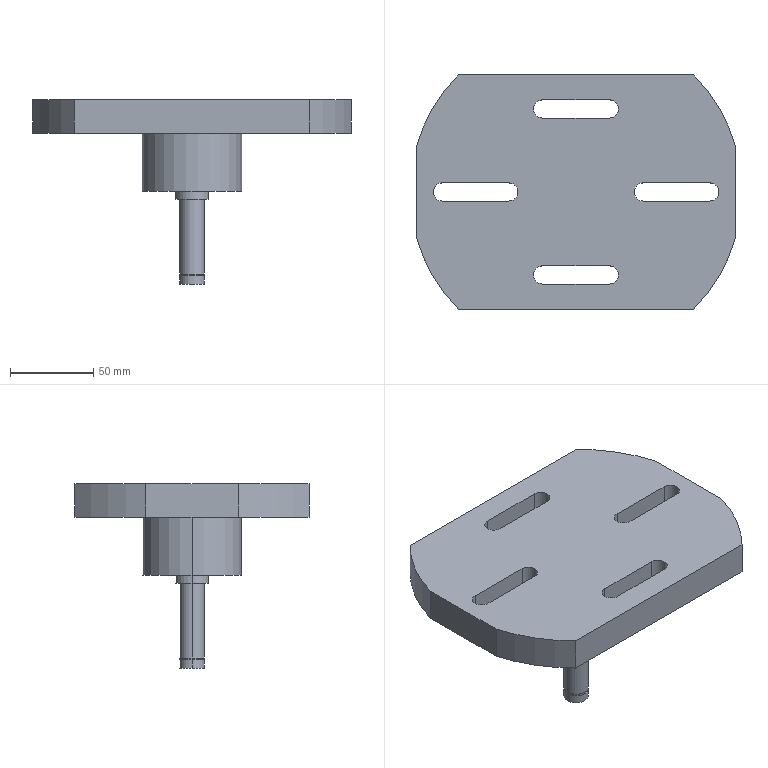Part | SolidWorks | features ICE 2, MirrorPattern 2, Revolution 1 | 1 solid | 45 faces | box 192 x 141 x 111 mm | volume 573691 mm3 | cylinder 26 | plane 19 | commonest cylinder face diameters 11 x12 15 x4 200 x4 14.3 x2 20 x2 60 x2
STEP:
#1=CARTESIAN_POINT('',(-20.,-44.5,0.));
#2=VERTEX_POINT('',#1);
#3=CARTESIAN_POINT('',(-25.5,-50.,0.));
#4=VERTEX_POINT('',#3);
#5=CARTESIAN_POINT('',(-20.,-50.,0.));
#6=DIRECTION('',(0.,0.,1.));
#7=DIRECTION('',(-1.,0.,0.));
#8=AXIS2_PLACEMENT_3D('',#5,#6,#7);
#9=CIRCLE('',#8,5.5);
#10=EDGE_CURVE('',#2,#4,#9,.T.);
#11=ORIENTED_EDGE('',*,*,#10,.T.);
#12=CARTESIAN_POINT('',(-25.5,-50.,-20.));
#13=VERTEX_POINT('',#12);
#14=CARTESIAN_POINT('',(-25.5,-50.,0.));
#15=DIRECTION('',(0.,0.,-1.));
#16=VECTOR('',#15,1000.);
#17=LINE('',#14,#16);
#18=EDGE_CURVE('',#4,#13,#17,.T.);
#19=ORIENTED_EDGE('',*,*,#18,.T.);
#20=CARTESIAN_POINT('',(-20.,-44.5,-20.));
#21=VERTEX_POINT('',#20);
#22=CARTESIAN_POINT('',(-20.,-50.,-20.));
#23=DIRECTION('',(0.,0.,1.));
#24=DIRECTION('',(-1.,0.,0.));
#25=AXIS2_PLACEMENT_3D('',#22,#23,#24);
#26=CIRCLE('',#25,5.5);
#27=EDGE_CURVE('',#21,#13,#26,.T.);
#28=ORIENTED_EDGE('',*,*,#27,.F.);
#29=CARTESIAN_POINT('',(-20.,-44.5,0.));
#30=DIRECTION('',(0.,0.,-1.));
#31=VECTOR('',#30,1000.);
#32=LINE('',#29,#31);
#33=EDGE_CURVE('',#2,#21,#32,.T.);
#34=ORIENTED_EDGE('',*,*,#33,.F.);
#35=EDGE_LOOP('',(#11,#19,#28,#34));
#36=FACE_OUTER_BOUND('',#35,.T.);
#37=CARTESIAN_POINT('',(-20.,-50.,0.));
#38=DIRECTION('',(0.,0.,-1.));
#39=DIRECTION('',(-1.,0.,0.));
#40=AXIS2_PLACEMENT_3D('',#37,#38,#39);
#41=CYLINDRICAL_SURFACE('',#40,5.5);
#42=ADVANCED_FACE('',(#36),#41,.F.);
#43=CARTESIAN_POINT('',(-80.5,5.5,0.));
#44=VERTEX_POINT('',#43);
#45=CARTESIAN_POINT('',(-86.,0.,0.));
#46=VERTEX_POINT('',#45);
#47=CARTESIAN_POINT('',(-80.5,0.,0.));
#48=DIRECTION('',(0.,0.,1.));
#49=DIRECTION('',(1.,0.,0.));
#50=AXIS2_PLACEMENT_3D('',#47,#48,#49);
#51=CIRCLE('',#50,5.5);
#52=EDGE_CURVE('',#44,#46,#51,.T.);
#53=ORIENTED_EDGE('',*,*,#52,.T.);
#54=CARTESIAN_POINT('',(-86.,0.,-20.));
#55=VERTEX_POINT('',#54);
#56=CARTESIAN_POINT('',(-86.,0.,0.));
#57=DIRECTION('',(0.,0.,-1.));
#58=VECTOR('',#57,1000.);
#59=LINE('',#56,#58);
#60=EDGE_CURVE('',#46,#55,#59,.T.);
#61=ORIENTED_EDGE('',*,*,#60,.T.);
#62=CARTESIAN_POINT('',(-80.5,5.5,-20.));
#63=VERTEX_POINT('',#62);
#64=CARTESIAN_POINT('',(-80.5,0.,-20.));
#65=DIRECTION('',(0.,0.,1.));
#66=DIRECTION('',(1.,0.,0.));
#67=AXIS2_PLACEMENT_3D('',#64,#65,#66);
#68=CIRCLE('',#67,5.5);
#69=EDGE_CURVE('',#63,#55,#68,.T.);
#70=ORIENTED_EDGE('',*,*,#69,.F.);
#71=CARTESIAN_POINT('',(-80.5,5.5,0.));
#72=DIRECTION('',(0.,0.,-1.));
#73=VECTOR('',#72,1000.);
#74=LINE('',#71,#73);
#75=EDGE_CURVE('',#44,#63,#74,.T.);
#76=ORIENTED_EDGE('',*,*,#75,.F.);
#77=EDGE_LOOP('',(#53,#61,#70,#76));
#78=FACE_OUTER_BOUND('',#77,.T.);
#79=CARTESIAN_POINT('',(-80.5,0.,0.));
#80=DIRECTION('',(0.,0.,-1.));
#81=DIRECTION('',(-1.,0.,0.));
#82=AXIS2_PLACEMENT_3D('',#79,#80,#81);
#83=CYLINDRICAL_SURFACE('',#82,5.5);
#84=ADVANCED_FACE('',(#78),#83,.F.);
#85=CARTESIAN_POINT('',(-25.5,50.,0.));
#86=VERTEX_POINT('',#85);
#87=CARTESIAN_POINT('',(-20.,55.5,0.));
#88=VERTEX_POINT('',#87);
#89=CARTESIAN_POINT('',(-20.,50.,0.));
#90=DIRECTION('',(0.,0.,-1.));
#91=DIRECTION('',(-1.,0.,0.));
#92=AXIS2_PLACEMENT_3D('',#89,#90,#91);
#93=CIRCLE('',#92,5.5);
#94=EDGE_CURVE('',#86,#88,#93,.T.);
#95=ORIENTED_EDGE('',*,*,#94,.F.);
#96=CARTESIAN_POINT('',(-25.5,50.,-20.));
#97=VERTEX_POINT('',#96);
#98=CARTESIAN_POINT('',(-25.5,50.,0.));
#99=DIRECTION('',(0.,0.,-1.));
#100=VECTOR('',#99,1000.);
#101=LINE('',#98,#100);
#102=EDGE_CURVE('',#86,#97,#101,.T.);
#103=ORIENTED_EDGE('',*,*,#102,.T.);
#104=CARTESIAN_POINT('',(-20.,55.5,-20.));
#105=VERTEX_POINT('',#104);
#106=CARTESIAN_POINT('',(-20.,50.,-20.));
#107=DIRECTION('',(0.,0.,-1.));
#108=DIRECTION('',(-1.,0.,0.));
#109=AXIS2_PLACEMENT_3D('',#106,#107,#108);
#110=CIRCLE('',#109,5.5);
#111=EDGE_CURVE('',#97,#105,#110,.T.);
#112=ORIENTED_EDGE('',*,*,#111,.T.);
#113=CARTESIAN_POINT('',(-20.,55.5,0.));
#114=DIRECTION('',(0.,0.,-1.));
#115=VECTOR('',#114,1000.);
#116=LINE('',#113,#115);
#117=EDGE_CURVE('',#88,#105,#116,.T.);
#118=ORIENTED_EDGE('',*,*,#117,.F.);
#119=EDGE_LOOP('',(#95,#103,#112,#118));
#120=FACE_OUTER_BOUND('',#119,.T.);
#121=CARTESIAN_POINT('',(-20.,50.,0.));
#122=DIRECTION('',(0.,0.,-1.));
#123=DIRECTION('',(-1.,0.,0.));
#124=AXIS2_PLACEMENT_3D('',#121,#122,#123);
#125=CYLINDRICAL_SURFACE('',#124,5.5);
#126=ADVANCED_FACE('',(#120),#125,.F.);
#127=CARTESIAN_POINT('',(35.,0.,0.));
#128=VERTEX_POINT('',#127);
#129=CARTESIAN_POINT('',(40.5,5.5,0.));
#130=VERTEX_POINT('',#129);
#131=CARTESIAN_POINT('',(40.5,0.,0.));
#132=DIRECTION('',(0.,0.,-1.));
#133=DIRECTION('',(-1.,0.,0.));
#134=AXIS2_PLACEMENT_3D('',#131,#132,#133);
#135=CIRCLE('',#134,5.5);
#136=EDGE_CURVE('',#128,#130,#135,.T.);
#137=ORIENTED_EDGE('',*,*,#136,.F.);
#138=CARTESIAN_POINT('',(35.,0.,-20.));
#139=VERTEX_POINT('',#138);
#140=CARTESIAN_POINT('',(35.,0.,0.));
#141=DIRECTION('',(0.,0.,-1.));
#142=VECTOR('',#141,1000.);
#143=LINE('',#140,#142);
#144=EDGE_CURVE('',#128,#139,#143,.T.);
#145=ORIENTED_EDGE('',*,*,#144,.T.);
#146=CARTESIAN_POINT('',(40.5,5.5,-20.));
#147=VERTEX_POINT('',#146);
#148=CARTESIAN_POINT('',(40.5,0.,-20.));
#149=DIRECTION('',(0.,0.,-1.));
#150=DIRECTION('',(-1.,0.,0.));
#151=AXIS2_PLACEMENT_3D('',#148,#149,#150);
#152=CIRCLE('',#151,5.5);
#153=EDGE_CURVE('',#139,#147,#152,.T.);
#154=ORIENTED_EDGE('',*,*,#153,.T.);
#155=CARTESIAN_POINT('',(40.5,5.5,0.));
#156=DIRECTION('',(0.,0.,-1.));
#157=VECTOR('',#156,1000.);
#158=LINE('',#155,#157);
#159=EDGE_CURVE('',#130,#147,#158,.T.);
#160=ORIENTED_EDGE('',*,*,#159,.F.);
#161=EDGE_LOOP('',(#137,#145,#154,#160));
#162=FACE_OUTER_BOUND('',#161,.T.);
#163=CARTESIAN_POINT('',(40.5,0.,0.));
#164=DIRECTION('',(0.,0.,-1.));
#165=DIRECTION('',(-1.,0.,0.));
#166=AXIS2_PLACEMENT_3D('',#163,#164,#165);
#167=CYLINDRICAL_SURFACE('',#166,5.5);
#168=ADVANCED_FACE('',(#162),#167,.F.);
#169=CARTESIAN_POINT('',(-30.,0.,-20.));
#170=VERTEX_POINT('',#169);
#171=CARTESIAN_POINT('',(30.,0.,-20.));
#172=VERTEX_POINT('',#171);
#173=CARTESIAN_POINT('',(0.,0.,-20.));
#174=DIRECTION('',(0.,0.,-1.));
#175=DIRECTION('',(-1.,0.,0.));
#176=AXIS2_PLACEMENT_3D('',#173,#174,#175);
#177=CIRCLE('',#176,30.);
#178=EDGE_CURVE('',#170,#172,#177,.T.);
#179=ORIENTED_EDGE('',*,*,#178,.T.);
#180=CARTESIAN_POINT('',(30.,0.,-55.));
#181=VERTEX_POINT('',#180);
#182=CARTESIAN_POINT('',(30.,0.,0.));
#183=DIRECTION('',(0.,0.,-1.));
#184=VECTOR('',#183,1000.);
#185=LINE('',#182,#184);
#186=EDGE_CURVE('',#172,#181,#185,.T.);
#187=ORIENTED_EDGE('',*,*,#186,.T.);
#188=CARTESIAN_POINT('',(-30.,0.,-55.));
#189=VERTEX_POINT('',#188);
#190=CARTESIAN_POINT('',(0.,0.,-55.));
#191=DIRECTION('',(0.,0.,-1.));
#192=DIRECTION('',(-1.,0.,0.));
#193=AXIS2_PLACEMENT_3D('',#190,#191,#192);
#194=CIRCLE('',#193,30.);
#195=EDGE_CURVE('',#189,#181,#194,.T.);
#196=ORIENTED_EDGE('',*,*,#195,.F.);
#197=CARTESIAN_POINT('',(-30.,0.,0.));
#198=DIRECTION('',(0.,0.,-1.));
#199=VECTOR('',#198,1000.);
#200=LINE('',#197,#199);
#201=EDGE_CURVE('',#170,#189,#200,.T.);
#202=ORIENTED_EDGE('',*,*,#201,.F.);
#203=EDGE_LOOP('',(#179,#187,#196,#202));
#204=FACE_OUTER_BOUND('',#203,.T.);
#205=CARTESIAN_POINT('',(0.,0.,0.));
#206=DIRECTION('',(0.,0.,-1.));
#207=DIRECTION('',(-1.,0.,0.));
#208=AXIS2_PLACEMENT_3D('',#205,#206,#207);
#209=CYLINDRICAL_SURFACE('',#208,30.);
#210=ADVANCED_FACE('',(#204),#209,.T.);
#211=CARTESIAN_POINT('',(-10.,0.,-55.));
#212=VERTEX_POINT('',#211);
#213=CARTESIAN_POINT('',(10.,0.,-55.));
#214=VERTEX_POINT('',#213);
#215=CARTESIAN_POINT('',(0.,0.,-55.));
#216=DIRECTION('',(0.,0.,-1.));
#217=DIRECTION('',(-1.,0.,0.));
#218=AXIS2_PLACEMENT_3D('',#215,#216,#217);
#219=CIRCLE('',#218,10.);
#220=EDGE_CURVE('',#212,#214,#219,.T.);
#221=ORIENTED_EDGE('',*,*,#220,.T.);
#222=CARTESIAN_POINT('',(10.,0.,-60.));
#223=VERTEX_POINT('',#222);
#224=CARTESIAN_POINT('',(10.,0.,0.));
#225=DIRECTION('',(0.,0.,-1.));
#226=VECTOR('',#225,1000.);
#227=LINE('',#224,#226);
#228=EDGE_CURVE('',#214,#223,#227,.T.);
#229=ORIENTED_EDGE('',*,*,#228,.T.);
#230=CARTESIAN_POINT('',(-10.,0.,-60.));
#231=VERTEX_POINT('',#230);
#232=CARTESIAN_POINT('',(0.,0.,-60.));
#233=DIRECTION('',(0.,0.,-1.));
#234=DIRECTION('',(-1.,0.,0.));
#235=AXIS2_PLACEMENT_3D('',#232,#233,#234);
#236=CIRCLE('',#235,10.);
#237=EDGE_CURVE('',#231,#223,#236,.T.);
#238=ORIENTED_EDGE('',*,*,#237,.F.);
#239=CARTESIAN_POINT('',(-10.,0.,0.));
#240=DIRECTION('',(0.,0.,-1.));
#241=VECTOR('',#240,1000.);
#242=LINE('',#239,#241);
#243=EDGE_CURVE('',#212,#231,#242,.T.);
#244=ORIENTED_EDGE('',*,*,#243,.F.);
#245=EDGE_LOOP('',(#221,#229,#238,#244));
#246=FACE_OUTER_BOUND('',#245,.T.);
#247=CARTESIAN_POINT('',(0.,0.,0.));
#248=DIRECTION('',(0.,0.,-1.));
#249=DIRECTION('',(-1.,0.,0.));
#250=AXIS2_PLACEMENT_3D('',#247,#248,#249);
#251=CYLINDRICAL_SURFACE('',#250,10.);
#252=ADVANCED_FACE('',(#246),#251,.T.);
#253=CARTESIAN_POINT('',(-7.5,0.,-60.));
#254=VERTEX_POINT('',#253);
#255=CARTESIAN_POINT('',(7.5,0.,-60.));
#256=VERTEX_POINT('',#255);
#257=CARTESIAN_POINT('',(0.,0.,-60.));
#258=DIRECTION('',(0.,0.,-1.));
#259=DIRECTION('',(-1.,0.,0.));
#260=AXIS2_PLACEMENT_3D('',#257,#258,#259);
#261=CIRCLE('',#260,7.5);
#262=EDGE_CURVE('',#254,#256,#261,.T.);
#263=ORIENTED_EDGE('',*,*,#262,.T.);
#264=CARTESIAN_POINT('',(7.5,0.,-104.9));
#265=VERTEX_POINT('',#264);
#266=CARTESIAN_POINT('',(7.5,0.,0.));
#267=DIRECTION('',(0.,0.,-1.));
#268=VECTOR('',#267,1000.);
#269=LINE('',#266,#268);
#270=EDGE_CURVE('',#256,#265,#269,.T.);
#271=ORIENTED_EDGE('',*,*,#270,.T.);
#272=CARTESIAN_POINT('',(-7.5,0.,-104.9));
#273=VERTEX_POINT('',#272);
#274=CARTESIAN_POINT('',(0.,0.,-104.9));
#275=DIRECTION('',(0.,0.,-1.));
#276=DIRECTION('',(-1.,0.,0.));
#277=AXIS2_PLACEMENT_3D('',#274,#275,#276);
#278=CIRCLE('',#277,7.5);
#279=EDGE_CURVE('',#273,#265,#278,.T.);
#280=ORIENTED_EDGE('',*,*,#279,.F.);
#281=CARTESIAN_POINT('',(-7.5,0.,0.));
#282=DIRECTION('',(0.,0.,-1.));
#283=VECTOR('',#282,1000.);
#284=LINE('',#281,#283);
#285=EDGE_CURVE('',#254,#273,#284,.T.);
#286=ORIENTED_EDGE('',*,*,#285,.F.);
#287=EDGE_LOOP('',(#263,#271,#280,#286));
#288=FACE_OUTER_BOUND('',#287,.T.);
#289=CARTESIAN_POINT('',(0.,0.,0.));
#290=DIRECTION('',(0.,0.,-1.));
#291=DIRECTION('',(-1.,0.,0.));
#292=AXIS2_PLACEMENT_3D('',#289,#290,#291);
#293=CYLINDRICAL_SURFACE('',#292,7.5);
#294=ADVANCED_FACE('',(#288),#293,.T.);
#295=CARTESIAN_POINT('',(-7.15,0.,-104.9));
#296=VERTEX_POINT('',#295);
#297=CARTESIAN_POINT('',(7.15,0.,-104.9));
#298=VERTEX_POINT('',#297);
#299=CARTESIAN_POINT('',(0.,0.,-104.9));
#300=DIRECTION('',(0.,0.,-1.));
#301=DIRECTION('',(-1.,0.,0.));
#302=AXIS2_PLACEMENT_3D('',#299,#300,#301);
#303=CIRCLE('',#302,7.15);
#304=EDGE_CURVE('',#296,#298,#303,.T.);
#305=ORIENTED_EDGE('',*,*,#304,.T.);
#306=CARTESIAN_POINT('',(7.15,0.,-106.));
#307=VERTEX_POINT('',#306);
#308=CARTESIAN_POINT('',(7.15,0.,0.));
#309=DIRECTION('',(0.,0.,-1.));
#310=VECTOR('',#309,1000.);
#311=LINE('',#308,#310);
#312=EDGE_CURVE('',#298,#307,#311,.T.);
#313=ORIENTED_EDGE('',*,*,#312,.T.);
#314=CARTESIAN_POINT('',(-7.15,0.,-106.));
#315=VERTEX_POINT('',#314);
#316=CARTESIAN_POINT('',(0.,0.,-106.));
#317=DIRECTION('',(0.,0.,-1.));
#318=DIRECTION('',(-1.,0.,0.));
#319=AXIS2_PLACEMENT_3D('',#316,#317,#318);
#320=CIRCLE('',#319,7.15);
#321=EDGE_CURVE('',#315,#307,#320,.T.);
#322=ORIENTED_EDGE('',*,*,#321,.F.);
#323=CARTESIAN_POINT('',(-7.15,0.,0.));
#324=DIRECTION('',(0.,0.,-1.));
#325=VECTOR('',#324,1000.);
#326=LINE('',#323,#325);
#327=EDGE_CURVE('',#296,#315,#326,.T.);
#328=ORIENTED_EDGE('',*,*,#327,.F.);
#329=EDGE_LOOP('',(#305,#313,#322,#328));
#330=FACE_OUTER_BOUND('',#329,.T.);
#331=CARTESIAN_POINT('',(0.,0.,0.));
#332=DIRECTION('',(0.,0.,-1.));
#333=DIRECTION('',(-1.,0.,0.));
#334=AXIS2_PLACEMENT_3D('',#331,#332,#333);
#335=CYLINDRICAL_SURFACE('',#334,7.15);
#336=ADVANCED_FACE('',(#330),#335,.T.);
#337=CARTESIAN_POINT('',(-7.5,0.,-106.));
#338=VERTEX_POINT('',#337);
#339=CARTESIAN_POINT('',(7.5,0.,-106.));
#340=VERTEX_POINT('',#339);
#341=CARTESIAN_POINT('',(0.,0.,-106.));
#342=DIRECTION('',(0.,0.,-1.));
#343=DIRECTION('',(-1.,0.,0.));
#344=AXIS2_PLACEMENT_3D('',#341,#342,#343);
#345=CIRCLE('',#344,7.5);
#346=EDGE_CURVE('',#338,#340,#345,.T.);
#347=ORIENTED_EDGE('',*,*,#346,.T.);
#348=CARTESIAN_POINT('',(7.5,0.,-111.));
#349=VERTEX_POINT('',#348);
#350=CARTESIAN_POINT('',(7.5,0.,0.));
#351=DIRECTION('',(0.,0.,-1.));
#352=VECTOR('',#351,1000.);
#353=LINE('',#350,#352);
#354=EDGE_CURVE('',#340,#349,#353,.T.);
#355=ORIENTED_EDGE('',*,*,#354,.T.);
#356=CARTESIAN_POINT('',(-7.5,0.,-111.));
#357=VERTEX_POINT('',#356);
#358=CARTESIAN_POINT('',(0.,0.,-111.));
#359=DIRECTION('',(0.,0.,-1.));
#360=DIRECTION('',(-1.,0.,0.));
#361=AXIS2_PLACEMENT_3D('',#358,#359,#360);
#362=CIRCLE('',#361,7.5);
#363=EDGE_CURVE('',#357,#349,#362,.T.);
#364=ORIENTED_EDGE('',*,*,#363,.F.);
#365=CARTESIAN_POINT('',(-7.5,0.,0.));
#366=DIRECTION('',(0.,0.,-1.));
#367=VECTOR('',#366,1000.);
#368=LINE('',#365,#367);
#369=EDGE_CURVE('',#338,#357,#368,.T.);
#370=ORIENTED_EDGE('',*,*,#369,.F.);
#371=EDGE_LOOP('',(#347,#355,#364,#370));
#372=FACE_OUTER_BOUND('',#371,.T.);
#373=CARTESIAN_POINT('',(0.,0.,0.));
#374=DIRECTION('',(0.,0.,-1.));
#375=DIRECTION('',(-1.,0.,0.));
#376=AXIS2_PLACEMENT_3D('',#373,#374,#375);
#377=CYLINDRICAL_SURFACE('',#376,7.5);
#378=ADVANCED_FACE('',(#372),#377,.T.);
#379=CARTESIAN_POINT('',(20.,55.5,-20.));
#380=VERTEX_POINT('',#379);
#381=CARTESIAN_POINT('',(20.,44.5,-20.));
#382=VERTEX_POINT('',#381);
#383=CARTESIAN_POINT('',(20.,50.,-20.));
#384=DIRECTION('',(0.,0.,-1.));
#385=DIRECTION('',(-1.,0.,0.));
#386=AXIS2_PLACEMENT_3D('',#383,#384,#385);
#387=CIRCLE('',#386,5.5);
#388=EDGE_CURVE('',#380,#382,#387,.T.);
#389=ORIENTED_EDGE('',*,*,#388,.F.);
#390=CARTESIAN_POINT('',(20.,55.5,-20.));
#391=DIRECTION('',(1.,0.,0.));
#392=VECTOR('',#391,1000.);
#393=LINE('',#390,#392);
#394=EDGE_CURVE('',#105,#380,#393,.T.);
#395=ORIENTED_EDGE('',*,*,#394,.F.);
#396=ORIENTED_EDGE('',*,*,#111,.F.);
#397=CARTESIAN_POINT('',(-20.,44.5,-20.));
#398=VERTEX_POINT('',#397);
#399=CARTESIAN_POINT('',(-20.,50.,-20.));
#400=DIRECTION('',(0.,0.,-1.));
#401=DIRECTION('',(-1.,0.,0.));
#402=AXIS2_PLACEMENT_3D('',#399,#400,#401);
#403=CIRCLE('',#402,5.5);
#404=EDGE_CURVE('',#398,#97,#403,.T.);
#405=ORIENTED_EDGE('',*,*,#404,.F.);
#406=CARTESIAN_POINT('',(20.,44.5,-20.));
#407=DIRECTION('',(-1.,0.,0.));
#408=VECTOR('',#407,1000.);
#409=LINE('',#406,#408);
#410=EDGE_CURVE('',#382,#398,#409,.T.);
#411=ORIENTED_EDGE('',*,*,#410,.F.);
#412=EDGE_LOOP('',(#389,#395,#396,#405,#411));
#413=FACE_BOUND('',#412,.T.);
#414=CARTESIAN_POINT('',(40.5,-5.5,-20.));
#415=VERTEX_POINT('',#414);
#416=CARTESIAN_POINT('',(40.5,0.,-20.));
#417=DIRECTION('',(0.,0.,-1.));
#418=DIRECTION('',(-1.,0.,0.));
#419=AXIS2_PLACEMENT_3D('',#416,#417,#418);
#420=CIRCLE('',#419,5.5);
#421=EDGE_CURVE('',#415,#139,#420,.T.);
#422=ORIENTED_EDGE('',*,*,#421,.F.);
#423=CARTESIAN_POINT('',(80.5,-5.5,-20.));
#424=VERTEX_POINT('',#423);
#425=CARTESIAN_POINT('',(40.5,-5.5,-20.));
#426=DIRECTION('',(-1.,0.,0.));
#427=VECTOR('',#426,1000.);
#428=LINE('',#425,#427);
#429=EDGE_CURVE('',#424,#415,#428,.T.);
#430=ORIENTED_EDGE('',*,*,#429,.F.);
#431=CARTESIAN_POINT('',(80.5,5.5,-20.));
#432=VERTEX_POINT('',#431);
#433=CARTESIAN_POINT('',(80.5,0.,-20.));
#434=DIRECTION('',(0.,0.,-1.));
#435=DIRECTION('',(-1.,0.,0.));
#436=AXIS2_PLACEMENT_3D('',#433,#434,#435);
#437=CIRCLE('',#436,5.5);
#438=EDGE_CURVE('',#432,#424,#437,.T.);
#439=ORIENTED_EDGE('',*,*,#438,.F.);
#440=CARTESIAN_POINT('',(40.5,5.5,-20.));
#441=DIRECTION('',(1.,0.,0.));
#442=VECTOR('',#441,1000.);
#443=LINE('',#440,#442);
#444=EDGE_CURVE('',#147,#432,#443,.T.);
#445=ORIENTED_EDGE('',*,*,#444,.F.);
#446=ORIENTED_EDGE('',*,*,#153,.F.);
#447=EDGE_LOOP('',(#422,#430,#439,#445,#446));
#448=FACE_BOUND('',#447,.T.);
#449=ORIENTED_EDGE('',*,*,#178,.F.);
#450=CARTESIAN_POINT('',(0.,0.,-20.));
#451=DIRECTION('',(0.,0.,-1.));
#452=DIRECTION('',(-1.,0.,0.));
#453=AXIS2_PLACEMENT_3D('',#450,#451,#452);
#454=CIRCLE('',#453,30.);
#455=EDGE_CURVE('',#172,#170,#454,.T.);
#456=ORIENTED_EDGE('',*,*,#455,.F.);
#457=EDGE_LOOP('',(#449,#456));
#458=FACE_BOUND('',#457,.T.);
#459=CARTESIAN_POINT('',(-80.5,-5.5,-20.));
#460=VERTEX_POINT('',#459);
#461=CARTESIAN_POINT('',(-40.5,-5.5,-20.));
#462=VERTEX_POINT('',#461);
#463=CARTESIAN_POINT('',(-40.5,-5.5,-20.));
#464=DIRECTION('',(1.,0.,0.));
#465=VECTOR('',#464,1000.);
#466=LINE('',#463,#465);
#467=EDGE_CURVE('',#460,#462,#466,.T.);
#468=ORIENTED_EDGE('',*,*,#467,.T.);
#469=CARTESIAN_POINT('',(-40.5,5.5,-20.));
#470=VERTEX_POINT('',#469);
#471=CARTESIAN_POINT('',(-40.5,0.,-20.));
#472=DIRECTION('',(0.,0.,1.));
#473=DIRECTION('',(1.,0.,0.));
#474=AXIS2_PLACEMENT_3D('',#471,#472,#473);
#475=CIRCLE('',#474,5.5);
#476=EDGE_CURVE('',#462,#470,#475,.T.);
#477=ORIENTED_EDGE('',*,*,#476,.T.);
#478=CARTESIAN_POINT('',(-40.5,5.5,-20.));
#479=DIRECTION('',(-1.,0.,0.));
#480=VECTOR('',#479,1000.);
#481=LINE('',#478,#480);
#482=EDGE_CURVE('',#470,#63,#481,.T.);
#483=ORIENTED_EDGE('',*,*,#482,.T.);
#484=ORIENTED_EDGE('',*,*,#69,.T.);
#485=CARTESIAN_POINT('',(-80.5,0.,-20.));
#486=DIRECTION('',(0.,0.,1.));
#487=DIRECTION('',(1.,0.,0.));
#488=AXIS2_PLACEMENT_3D('',#485,#486,#487);
#489=CIRCLE('',#488,5.5);
#490=EDGE_CURVE('',#55,#460,#489,.T.);
#491=ORIENTED_EDGE('',*,*,#490,.T.);
#492=EDGE_LOOP('',(#468,#477,#483,#484,#491));
#493=FACE_BOUND('',#492,.T.);
#494=CARTESIAN_POINT('',(-20.,-55.5,-20.));
#495=VERTEX_POINT('',#494);
#496=CARTESIAN_POINT('',(20.,-55.5,-20.));
#497=VERTEX_POINT('',#496);
#498=CARTESIAN_POINT('',(20.,-55.5,-20.));
#499=DIRECTION('',(1.,0.,0.));
#500=VECTOR('',#499,1000.);
#501=LINE('',#498,#500);
#502=EDGE_CURVE('',#495,#497,#501,.T.);
#503=ORIENTED_EDGE('',*,*,#502,.T.);
#504=CARTESIAN_POINT('',(20.,-44.5,-20.));
#505=VERTEX_POINT('',#504);
#506=CARTESIAN_POINT('',(20.,-50.,-20.));
#507=DIRECTION('',(0.,0.,1.));
#508=DIRECTION('',(-1.,0.,0.));
#509=AXIS2_PLACEMENT_3D('',#506,#507,#508);
#510=CIRCLE('',#509,5.5);
#511=EDGE_CURVE('',#497,#505,#510,.T.);
#512=ORIENTED_EDGE('',*,*,#511,.T.);
#513=CARTESIAN_POINT('',(20.,-44.5,-20.));
#514=DIRECTION('',(-1.,0.,0.));
#515=VECTOR('',#514,1000.);
#516=LINE('',#513,#515);
#517=EDGE_CURVE('',#505,#21,#516,.T.);
#518=ORIENTED_EDGE('',*,*,#517,.T.);
#519=ORIENTED_EDGE('',*,*,#27,.T.);
#520=CARTESIAN_POINT('',(-20.,-50.,-20.));
#521=DIRECTION('',(0.,0.,1.));
#522=DIRECTION('',(-1.,0.,0.));
#523=AXIS2_PLACEMENT_3D('',#520,#521,#522);
#524=CIRCLE('',#523,5.5);
#525=EDGE_CURVE('',#13,#495,#524,.T.);
#526=ORIENTED_EDGE('',*,*,#525,.T.);
#527=EDGE_LOOP('',(#503,#512,#518,#519,#526));
#528=FACE_BOUND('',#527,.T.);
#529=CARTESIAN_POINT('',(-70.921,-70.5,-20.));
#530=VERTEX_POINT('',#529);
#531=CARTESIAN_POINT('',(-96.,-28.,-20.));
#532=VERTEX_POINT('',#531);
#533=CARTESIAN_POINT('',(0.,0.,-20.));
#534=DIRECTION('',(0.,0.,-1.));
#535=DIRECTION('',(-1.,0.,0.));
#536=AXIS2_PLACEMENT_3D('',#533,#534,#535);
#537=CIRCLE('',#536,100.);
#538=EDGE_CURVE('',#530,#532,#537,.T.);
#539=ORIENTED_EDGE('',*,*,#538,.T.);
#540=CARTESIAN_POINT('',(-96.,28.,-20.));
#541=VERTEX_POINT('',#540);
#542=CARTESIAN_POINT('',(-96.,-70.5,-20.));
#543=DIRECTION('',(0.,1.,0.));
#544=VECTOR('',#543,1000.);
#545=LINE('',#542,#544);
#546=EDGE_CURVE('',#532,#541,#545,.T.);
#547=ORIENTED_EDGE('',*,*,#546,.T.);
#548=CARTESIAN_POINT('',(-70.921,70.5,-20.));
#549=VERTEX_POINT('',#548);
#550=CARTESIAN_POINT('',(0.,0.,-20.));
#551=DIRECTION('',(0.,0.,-1.));
#552=DIRECTION('',(-1.,0.,0.));
#553=AXIS2_PLACEMENT_3D('',#550,#551,#552);
#554=CIRCLE('',#553,100.);
#555=EDGE_CURVE('',#541,#549,#554,.T.);
#556=ORIENTED_EDGE('',*,*,#555,.T.);
#557=CARTESIAN_POINT('',(70.921,70.5,-20.));
#558=VERTEX_POINT('',#557);
#559=CARTESIAN_POINT('',(96.,70.5,-20.));
#560=DIRECTION('',(1.,0.,0.));
#561=VECTOR('',#560,1000.);
#562=LINE('',#559,#561);
#563=EDGE_CURVE('',#549,#558,#562,.T.);
#564=ORIENTED_EDGE('',*,*,#563,.T.);
#565=CARTESIAN_POINT('',(96.,28.,-20.));
#566=VERTEX_POINT('',#565);
#567=CARTESIAN_POINT('',(0.,0.,-20.));
#568=DIRECTION('',(0.,0.,-1.));
#569=DIRECTION('',(-1.,0.,0.));
#570=AXIS2_PLACEMENT_3D('',#567,#568,#569);
#571=CIRCLE('',#570,100.);
#572=EDGE_CURVE('',#558,#566,#571,.T.);
#573=ORIENTED_EDGE('',*,*,#572,.T.);
#574=CARTESIAN_POINT('',(96.,-28.,-20.));
#575=VERTEX_POINT('',#574);
#576=CARTESIAN_POINT('',(96.,-70.5,-20.));
#577=DIRECTION('',(0.,-1.,0.));
#578=VECTOR('',#577,1000.);
#579=LINE('',#576,#578);
#580=EDGE_CURVE('',#566,#575,#579,.T.);
#581=ORIENTED_EDGE('',*,*,#580,.T.);
#582=CARTESIAN_POINT('',(70.921,-70.5,-20.));
#583=VERTEX_POINT('',#582);
#584=CARTESIAN_POINT('',(0.,0.,-20.));
#585=DIRECTION('',(0.,0.,-1.));
#586=DIRECTION('',(-1.,0.,0.));
#587=AXIS2_PLACEMENT_3D('',#584,#585,#586);
#588=CIRCLE('',#587,100.);
#589=EDGE_CURVE('',#575,#583,#588,.T.);
#590=ORIENTED_EDGE('',*,*,#589,.T.);
#591=CARTESIAN_POINT('',(96.,-70.5,-20.));
#592=DIRECTION('',(-1.,0.,0.));
#593=VECTOR('',#592,1000.);
#594=LINE('',#591,#593);
#595=EDGE_CURVE('',#583,#530,#594,.T.);
#596=ORIENTED_EDGE('',*,*,#595,.T.);
#597=EDGE_LOOP('',(#539,#547,#556,#564,#573,#581,#590,#596));
#598=FACE_OUTER_BOUND('',#597,.T.);
#599=CARTESIAN_POINT('',(-30.,0.,-20.));
#600=DIRECTION('',(0.,0.,-1.));
#601=DIRECTION('',(-1.,0.,0.));
#602=AXIS2_PLACEMENT_3D('',#599,#600,#601);
#603=PLANE('',#602);
#604=ADVANCED_FACE('',(#413,#448,#458,#493,#528,#598),#603,.T.);
#605=CARTESIAN_POINT('',(20.,55.5,0.));
#606=VERTEX_POINT('',#605);
#607=CARTESIAN_POINT('',(20.,44.5,0.));
#608=VERTEX_POINT('',#607);
#609=CARTESIAN_POINT('',(20.,50.,0.));
#610=DIRECTION('',(0.,0.,-1.));
#611=DIRECTION('',(-1.,0.,0.));
#612=AXIS2_PLACEMENT_3D('',#609,#610,#611);
#613=CIRCLE('',#612,5.5);
#614=EDGE_CURVE('',#606,#608,#613,.T.);
#615=ORIENTED_EDGE('',*,*,#614,.T.);
#616=CARTESIAN_POINT('',(-20.,44.5,0.));
#617=VERTEX_POINT('',#616);
#618=CARTESIAN_POINT('',(20.,44.5,0.));
#619=DIRECTION('',(-1.,0.,0.));
#620=VECTOR('',#619,1000.);
#621=LINE('',#618,#620);
#622=EDGE_CURVE('',#608,#617,#621,.T.);
#623=ORIENTED_EDGE('',*,*,#622,.T.);
#624=CARTESIAN_POINT('',(-20.,50.,0.));
#625=DIRECTION('',(0.,0.,-1.));
#626=DIRECTION('',(-1.,0.,0.));
#627=AXIS2_PLACEMENT_3D('',#624,#625,#626);
#628=CIRCLE('',#627,5.5);
#629=EDGE_CURVE('',#617,#86,#628,.T.);
#630=ORIENTED_EDGE('',*,*,#629,.T.);
#631=ORIENTED_EDGE('',*,*,#94,.T.);
#632=CARTESIAN_POINT('',(20.,55.5,0.));
#633=DIRECTION('',(1.,0.,0.));
#634=VECTOR('',#633,1000.);
#635=LINE('',#632,#634);
#636=EDGE_CURVE('',#88,#606,#635,.T.);
#637=ORIENTED_EDGE('',*,*,#636,.T.);
#638=EDGE_LOOP('',(#615,#623,#630,#631,#637));
#639=FACE_BOUND('',#638,.T.);
#640=CARTESIAN_POINT('',(40.5,-5.5,0.));
#641=VERTEX_POINT('',#640);
#642=CARTESIAN_POINT('',(40.5,0.,0.));
#643=DIRECTION('',(0.,0.,-1.));
#644=DIRECTION('',(-1.,0.,0.));
#645=AXIS2_PLACEMENT_3D('',#642,#643,#644);
#646=CIRCLE('',#645,5.5);
#647=EDGE_CURVE('',#641,#128,#646,.T.);
#648=ORIENTED_EDGE('',*,*,#647,.T.);
#649=ORIENTED_EDGE('',*,*,#136,.T.);
#650=CARTESIAN_POINT('',(80.5,5.5,0.));
#651=VERTEX_POINT('',#650);
#652=CARTESIAN_POINT('',(40.5,5.5,0.));
#653=DIRECTION('',(1.,0.,0.));
#654=VECTOR('',#653,1000.);
#655=LINE('',#652,#654);
#656=EDGE_CURVE('',#130,#651,#655,.T.);
#657=ORIENTED_EDGE('',*,*,#656,.T.);
#658=CARTESIAN_POINT('',(80.5,-5.5,0.));
#659=VERTEX_POINT('',#658);
#660=CARTESIAN_POINT('',(80.5,0.,0.));
#661=DIRECTION('',(0.,0.,-1.));
#662=DIRECTION('',(-1.,0.,0.));
#663=AXIS2_PLACEMENT_3D('',#660,#661,#662);
#664=CIRCLE('',#663,5.5);
#665=EDGE_CURVE('',#651,#659,#664,.T.);
#666=ORIENTED_EDGE('',*,*,#665,.T.);
#667=CARTESIAN_POINT('',(40.5,-5.5,0.));
#668=DIRECTION('',(-1.,0.,0.));
#669=VECTOR('',#668,1000.);
#670=LINE('',#667,#669);
#671=EDGE_CURVE('',#659,#641,#670,.T.);
#672=ORIENTED_EDGE('',*,*,#671,.T.);
#673=EDGE_LOOP('',(#648,#649,#657,#666,#672));
#674=FACE_BOUND('',#673,.T.);
#675=CARTESIAN_POINT('',(-40.5,5.5,0.));
#676=VERTEX_POINT('',#675);
#677=CARTESIAN_POINT('',(-40.5,5.5,0.));
#678=DIRECTION('',(-1.,0.,0.));
#679=VECTOR('',#678,1000.);
#680=LINE('',#677,#679);
#681=EDGE_CURVE('',#676,#44,#680,.T.);
#682=ORIENTED_EDGE('',*,*,#681,.F.);
#683=CARTESIAN_POINT('',(-40.5,-5.5,0.));
#684=VERTEX_POINT('',#683);
#685=CARTESIAN_POINT('',(-40.5,0.,0.));
#686=DIRECTION('',(0.,0.,1.));
#687=DIRECTION('',(1.,0.,0.));
#688=AXIS2_PLACEMENT_3D('',#685,#686,#687);
#689=CIRCLE('',#688,5.5);
#690=EDGE_CURVE('',#684,#676,#689,.T.);
#691=ORIENTED_EDGE('',*,*,#690,.F.);
#692=CARTESIAN_POINT('',(-80.5,-5.5,0.));
#693=VERTEX_POINT('',#692);
#694=CARTESIAN_POINT('',(-40.5,-5.5,0.));
#695=DIRECTION('',(1.,0.,0.));
#696=VECTOR('',#695,1000.);
#697=LINE('',#694,#696);
#698=EDGE_CURVE('',#693,#684,#697,.T.);
#699=ORIENTED_EDGE('',*,*,#698,.F.);
#700=CARTESIAN_POINT('',(-80.5,0.,0.));
#701=DIRECTION('',(0.,0.,1.));
#702=DIRECTION('',(1.,0.,0.));
#703=AXIS2_PLACEMENT_3D('',#700,#701,#702);
#704=CIRCLE('',#703,5.5);
#705=EDGE_CURVE('',#46,#693,#704,.T.);
#706=ORIENTED_EDGE('',*,*,#705,.F.);
#707=ORIENTED_EDGE('',*,*,#52,.F.);
#708=EDGE_LOOP('',(#682,#691,#699,#706,#707));
#709=FACE_BOUND('',#708,.T.);
#710=CARTESIAN_POINT('',(20.,-44.5,0.));
#711=VERTEX_POINT('',#710);
#712=CARTESIAN_POINT('',(20.,-44.5,0.));
#713=DIRECTION('',(-1.,0.,0.));
#714=VECTOR('',#713,1000.);
#715=LINE('',#712,#714);
#716=EDGE_CURVE('',#711,#2,#715,.T.);
#717=ORIENTED_EDGE('',*,*,#716,.F.);
#718=CARTESIAN_POINT('',(20.,-55.5,0.));
#719=VERTEX_POINT('',#718);
#720=CARTESIAN_POINT('',(20.,-50.,0.));
#721=DIRECTION('',(0.,0.,1.));
#722=DIRECTION('',(-1.,0.,0.));
#723=AXIS2_PLACEMENT_3D('',#720,#721,#722);
#724=CIRCLE('',#723,5.5);
#725=EDGE_CURVE('',#719,#711,#724,.T.);
#726=ORIENTED_EDGE('',*,*,#725,.F.);
#727=CARTESIAN_POINT('',(-20.,-55.5,0.));
#728=VERTEX_POINT('',#727);
#729=CARTESIAN_POINT('',(20.,-55.5,0.));
#730=DIRECTION('',(1.,0.,0.));
#731=VECTOR('',#730,1000.);
#732=LINE('',#729,#731);
#733=EDGE_CURVE('',#728,#719,#732,.T.);
#734=ORIENTED_EDGE('',*,*,#733,.F.);
#735=CARTESIAN_POINT('',(-20.,-50.,0.));
#736=DIRECTION('',(0.,0.,1.));
#737=DIRECTION('',(-1.,0.,0.));
#738=AXIS2_PLACEMENT_3D('',#735,#736,#737);
#739=CIRCLE('',#738,5.5);
#740=EDGE_CURVE('',#4,#728,#739,.T.);
#741=ORIENTED_EDGE('',*,*,#740,.F.);
#742=ORIENTED_EDGE('',*,*,#10,.F.);
#743=EDGE_LOOP('',(#717,#726,#734,#741,#742));
#744=FACE_BOUND('',#743,.T.);
#745=CARTESIAN_POINT('',(-96.,28.,0.));
#746=VERTEX_POINT('',#745);
#747=CARTESIAN_POINT('',(-70.921,70.5,0.));
#748=VERTEX_POINT('',#747);
#749=CARTESIAN_POINT('',(0.,0.,0.));
#750=DIRECTION('',(0.,0.,-1.));
#751=DIRECTION('',(-1.,0.,0.));
#752=AXIS2_PLACEMENT_3D('',#749,#750,#751);
#753=CIRCLE('',#752,100.);
#754=EDGE_CURVE('',#746,#748,#753,.T.);
#755=ORIENTED_EDGE('',*,*,#754,.F.);
#756=CARTESIAN_POINT('',(-96.,-28.,0.));
#757=VERTEX_POINT('',#756);
#758=CARTESIAN_POINT('',(-96.,-70.5,0.));
#759=DIRECTION('',(0.,1.,0.));
#760=VECTOR('',#759,1000.);
#761=LINE('',#758,#760);
#762=EDGE_CURVE('',#757,#746,#761,.T.);
#763=ORIENTED_EDGE('',*,*,#762,.F.);
#764=CARTESIAN_POINT('',(-70.921,-70.5,0.));
#765=VERTEX_POINT('',#764);
#766=CARTESIAN_POINT('',(0.,0.,0.));
#767=DIRECTION('',(0.,0.,-1.));
#768=DIRECTION('',(-1.,0.,0.));
#769=AXIS2_PLACEMENT_3D('',#766,#767,#768);
#770=CIRCLE('',#769,100.);
#771=EDGE_CURVE('',#765,#757,#770,.T.);
#772=ORIENTED_EDGE('',*,*,#771,.F.);
#773=CARTESIAN_POINT('',(70.921,-70.5,0.));
#774=VERTEX_POINT('',#773);
#775=CARTESIAN_POINT('',(96.,-70.5,0.));
#776=DIRECTION('',(-1.,0.,0.));
#777=VECTOR('',#776,1000.);
#778=LINE('',#775,#777);
#779=EDGE_CURVE('',#774,#765,#778,.T.);
#780=ORIENTED_EDGE('',*,*,#779,.F.);
#781=CARTESIAN_POINT('',(96.,-28.,0.));
#782=VERTEX_POINT('',#781);
#783=CARTESIAN_POINT('',(0.,0.,0.));
#784=DIRECTION('',(0.,0.,-1.));
#785=DIRECTION('',(-1.,0.,0.));
#786=AXIS2_PLACEMENT_3D('',#783,#784,#785);
#787=CIRCLE('',#786,100.);
#788=EDGE_CURVE('',#782,#774,#787,.T.);
#789=ORIENTED_EDGE('',*,*,#788,.F.);
#790=CARTESIAN_POINT('',(96.,28.,0.));
#791=VERTEX_POINT('',#790);
#792=CARTESIAN_POINT('',(96.,-70.5,0.));
#793=DIRECTION('',(0.,-1.,0.));
#794=VECTOR('',#793,1000.);
#795=LINE('',#792,#794);
#796=EDGE_CURVE('',#791,#782,#795,.T.);
#797=ORIENTED_EDGE('',*,*,#796,.F.);
#798=CARTESIAN_POINT('',(70.921,70.5,0.));
#799=VERTEX_POINT('',#798);
#800=CARTESIAN_POINT('',(0.,0.,0.));
#801=DIRECTION('',(0.,0.,-1.));
#802=DIRECTION('',(-1.,0.,0.));
#803=AXIS2_PLACEMENT_3D('',#800,#801,#802);
#804=CIRCLE('',#803,100.);
#805=EDGE_CURVE('',#799,#791,#804,.T.);
#806=ORIENTED_EDGE('',*,*,#805,.F.);
#807=CARTESIAN_POINT('',(96.,70.5,0.));
#808=DIRECTION('',(1.,0.,0.));
#809=VECTOR('',#808,1000.);
#810=LINE('',#807,#809);
#811=EDGE_CURVE('',#748,#799,#810,.T.);
#812=ORIENTED_EDGE('',*,*,#811,.F.);
#813=EDGE_LOOP('',(#755,#763,#772,#780,#789,#797,#806,#812));
#814=FACE_OUTER_BOUND('',#813,.T.);
#815=CARTESIAN_POINT('',(-100.,0.,0.));
#816=DIRECTION('',(0.,0.,1.));
#817=DIRECTION('',(1.,0.,0.));
#818=AXIS2_PLACEMENT_3D('',#815,#816,#817);
#819=PLANE('',#818);
#820=ADVANCED_FACE('',(#639,#674,#709,#744,#814),#819,.T.);
#821=ORIENTED_EDGE('',*,*,#555,.F.);
#822=CARTESIAN_POINT('',(-96.,28.,0.));
#823=DIRECTION('',(0.,0.,1.));
#824=VECTOR('',#823,1000.);
#825=LINE('',#822,#824);
#826=EDGE_CURVE('',#541,#746,#825,.T.);
#827=ORIENTED_EDGE('',*,*,#826,.T.);
#828=ORIENTED_EDGE('',*,*,#754,.T.);
#829=CARTESIAN_POINT('',(-70.921,70.5,0.));
#830=DIRECTION('',(0.,0.,-1.));
#831=VECTOR('',#830,1000.);
#832=LINE('',#829,#831);
#833=EDGE_CURVE('',#748,#549,#832,.T.);
#834=ORIENTED_EDGE('',*,*,#833,.T.);
#835=EDGE_LOOP('',(#821,#827,#828,#834));
#836=FACE_OUTER_BOUND('',#835,.T.);
#837=CARTESIAN_POINT('',(0.,0.,0.));
#838=DIRECTION('',(0.,0.,-1.));
#839=DIRECTION('',(-1.,0.,0.));
#840=AXIS2_PLACEMENT_3D('',#837,#838,#839);
#841=CYLINDRICAL_SURFACE('',#840,100.);
#842=ADVANCED_FACE('',(#836),#841,.T.);
#843=ORIENTED_EDGE('',*,*,#771,.T.);
#844=CARTESIAN_POINT('',(-96.,-28.,0.));
#845=DIRECTION('',(0.,0.,-1.));
#846=VECTOR('',#845,1000.);
#847=LINE('',#844,#846);
#848=EDGE_CURVE('',#757,#532,#847,.T.);
#849=ORIENTED_EDGE('',*,*,#848,.T.);
#850=ORIENTED_EDGE('',*,*,#538,.F.);
#851=CARTESIAN_POINT('',(-70.921,-70.5,0.));
#852=DIRECTION('',(0.,0.,1.));
#853=VECTOR('',#852,1000.);
#854=LINE('',#851,#853);
#855=EDGE_CURVE('',#530,#765,#854,.T.);
#856=ORIENTED_EDGE('',*,*,#855,.T.);
#857=EDGE_LOOP('',(#843,#849,#850,#856));
#858=FACE_OUTER_BOUND('',#857,.T.);
#859=CARTESIAN_POINT('',(0.,0.,0.));
#860=DIRECTION('',(0.,0.,-1.));
#861=DIRECTION('',(-1.,0.,0.));
#862=AXIS2_PLACEMENT_3D('',#859,#860,#861);
#863=CYLINDRICAL_SURFACE('',#862,100.);
#864=ADVANCED_FACE('',(#858),#863,.T.);
#865=ORIENTED_EDGE('',*,*,#788,.T.);
#866=CARTESIAN_POINT('',(70.921,-70.5,0.));
#867=DIRECTION('',(0.,0.,-1.));
#868=VECTOR('',#867,1000.);
#869=LINE('',#866,#868);
#870=EDGE_CURVE('',#774,#583,#869,.T.);
#871=ORIENTED_EDGE('',*,*,#870,.T.);
#872=ORIENTED_EDGE('',*,*,#589,.F.);
#873=CARTESIAN_POINT('',(96.,-28.,0.));
#874=DIRECTION('',(0.,0.,1.));
#875=VECTOR('',#874,1000.);
#876=LINE('',#873,#875);
#877=EDGE_CURVE('',#575,#782,#876,.T.);
#878=ORIENTED_EDGE('',*,*,#877,.T.);
#879=EDGE_LOOP('',(#865,#871,#872,#878));
#880=FACE_OUTER_BOUND('',#879,.T.);
#881=CARTESIAN_POINT('',(0.,0.,0.));
#882=DIRECTION('',(0.,0.,-1.));
#883=DIRECTION('',(-1.,0.,0.));
#884=AXIS2_PLACEMENT_3D('',#881,#882,#883);
#885=CYLINDRICAL_SURFACE('',#884,100.);
#886=ADVANCED_FACE('',(#880),#885,.T.);
#887=ORIENTED_EDGE('',*,*,#805,.T.);
#888=CARTESIAN_POINT('',(96.,28.,0.));
#889=DIRECTION('',(0.,0.,-1.));
#890=VECTOR('',#889,1000.);
#891=LINE('',#888,#890);
#892=EDGE_CURVE('',#791,#566,#891,.T.);
#893=ORIENTED_EDGE('',*,*,#892,.T.);
#894=ORIENTED_EDGE('',*,*,#572,.F.);
#895=CARTESIAN_POINT('',(70.921,70.5,0.));
#896=DIRECTION('',(0.,0.,1.));
#897=VECTOR('',#896,1000.);
#898=LINE('',#895,#897);
#899=EDGE_CURVE('',#558,#799,#898,.T.);
#900=ORIENTED_EDGE('',*,*,#899,.T.);
#901=EDGE_LOOP('',(#887,#893,#894,#900));
#902=FACE_OUTER_BOUND('',#901,.T.);
#903=CARTESIAN_POINT('',(0.,0.,0.));
#904=DIRECTION('',(0.,0.,-1.));
#905=DIRECTION('',(-1.,0.,0.));
#906=AXIS2_PLACEMENT_3D('',#903,#904,#905);
#907=CYLINDRICAL_SURFACE('',#906,100.);
#908=ADVANCED_FACE('',(#902),#907,.T.);
#909=ORIENTED_EDGE('',*,*,#363,.T.);
#910=CARTESIAN_POINT('',(0.,0.,-111.));
#911=DIRECTION('',(0.,0.,-1.));
#912=DIRECTION('',(-1.,0.,0.));
#913=AXIS2_PLACEMENT_3D('',#910,#911,#912);
#914=CIRCLE('',#913,7.5);
#915=EDGE_CURVE('',#349,#357,#914,.T.);
#916=ORIENTED_EDGE('',*,*,#915,.T.);
#917=EDGE_LOOP('',(#909,#916));
#918=FACE_OUTER_BOUND('',#917,.T.);
#919=CARTESIAN_POINT('',(0.,0.,-111.));
#920=DIRECTION('',(0.,0.,-1.));
#921=DIRECTION('',(-1.,0.,0.));
#922=AXIS2_PLACEMENT_3D('',#919,#920,#921);
#923=PLANE('',#922);
#924=ADVANCED_FACE('',(#918),#923,.T.);
#925=ORIENTED_EDGE('',*,*,#354,.F.);
#926=CARTESIAN_POINT('',(0.,0.,-106.));
#927=DIRECTION('',(0.,0.,-1.));
#928=DIRECTION('',(-1.,0.,0.));
#929=AXIS2_PLACEMENT_3D('',#926,#927,#928);
#930=CIRCLE('',#929,7.5);
#931=EDGE_CURVE('',#340,#338,#930,.T.);
#932=ORIENTED_EDGE('',*,*,#931,.T.);
#933=ORIENTED_EDGE('',*,*,#369,.T.);
#934=ORIENTED_EDGE('',*,*,#915,.F.);
#935=EDGE_LOOP('',(#925,#932,#933,#934));
#936=FACE_OUTER_BOUND('',#935,.T.);
#937=CARTESIAN_POINT('',(0.,0.,0.));
#938=DIRECTION('',(0.,0.,-1.));
#939=DIRECTION('',(-1.,0.,0.));
#940=AXIS2_PLACEMENT_3D('',#937,#938,#939);
#941=CYLINDRICAL_SURFACE('',#940,7.5);
#942=ADVANCED_FACE('',(#936),#941,.T.);
#943=ORIENTED_EDGE('',*,*,#321,.T.);
#944=CARTESIAN_POINT('',(0.,0.,-106.));
#945=DIRECTION('',(0.,0.,-1.));
#946=DIRECTION('',(-1.,0.,0.));
#947=AXIS2_PLACEMENT_3D('',#944,#945,#946);
#948=CIRCLE('',#947,7.15);
#949=EDGE_CURVE('',#307,#315,#948,.T.);
#950=ORIENTED_EDGE('',*,*,#949,.T.);
#951=EDGE_LOOP('',(#943,#950));
#952=FACE_BOUND('',#951,.T.);
#953=ORIENTED_EDGE('',*,*,#346,.F.);
#954=ORIENTED_EDGE('',*,*,#931,.F.);
#955=EDGE_LOOP('',(#953,#954));
#956=FACE_OUTER_BOUND('',#955,.T.);
#957=CARTESIAN_POINT('',(-7.5,0.,-106.));
#958=DIRECTION('',(0.,0.,1.));
#959=DIRECTION('',(1.,0.,0.));
#960=AXIS2_PLACEMENT_3D('',#957,#958,#959);
#961=PLANE('',#960);
#962=ADVANCED_FACE('',(#952,#956),#961,.T.);
#963=ORIENTED_EDGE('',*,*,#312,.F.);
#964=CARTESIAN_POINT('',(0.,0.,-104.9));
#965=DIRECTION('',(0.,0.,-1.));
#966=DIRECTION('',(-1.,0.,0.));
#967=AXIS2_PLACEMENT_3D('',#964,#965,#966);
#968=CIRCLE('',#967,7.15);
#969=EDGE_CURVE('',#298,#296,#968,.T.);
#970=ORIENTED_EDGE('',*,*,#969,.T.);
#971=ORIENTED_EDGE('',*,*,#327,.T.);
#972=ORIENTED_EDGE('',*,*,#949,.F.);
#973=EDGE_LOOP('',(#963,#970,#971,#972));
#974=FACE_OUTER_BOUND('',#973,.T.);
#975=CARTESIAN_POINT('',(0.,0.,0.));
#976=DIRECTION('',(0.,0.,-1.));
#977=DIRECTION('',(-1.,0.,0.));
#978=AXIS2_PLACEMENT_3D('',#975,#976,#977);
#979=CYLINDRICAL_SURFACE('',#978,7.15);
#980=ADVANCED_FACE('',(#974),#979,.T.);
#981=ORIENTED_EDGE('',*,*,#279,.T.);
#982=CARTESIAN_POINT('',(0.,0.,-104.9));
#983=DIRECTION('',(0.,0.,-1.));
#984=DIRECTION('',(-1.,0.,0.));
#985=AXIS2_PLACEMENT_3D('',#982,#983,#984);
#986=CIRCLE('',#985,7.5);
#987=EDGE_CURVE('',#265,#273,#986,.T.);
#988=ORIENTED_EDGE('',*,*,#987,.T.);
#989=EDGE_LOOP('',(#981,#988));
#990=FACE_OUTER_BOUND('',#989,.T.);
#991=ORIENTED_EDGE('',*,*,#304,.F.);
#992=ORIENTED_EDGE('',*,*,#969,.F.);
#993=EDGE_LOOP('',(#991,#992));
#994=FACE_BOUND('',#993,.T.);
#995=CARTESIAN_POINT('',(-7.15,0.,-104.9));
#996=DIRECTION('',(0.,0.,-1.));
#997=DIRECTION('',(-1.,0.,0.));
#998=AXIS2_PLACEMENT_3D('',#995,#996,#997);
#999=PLANE('',#998);
#1000=ADVANCED_FACE('',(#990,#994),#999,.T.);
#1001=ORIENTED_EDGE('',*,*,#270,.F.);
#1002=CARTESIAN_POINT('',(0.,0.,-60.));
#1003=DIRECTION('',(0.,0.,-1.));
#1004=DIRECTION('',(-1.,0.,0.));
#1005=AXIS2_PLACEMENT_3D('',#1002,#1003,#1004);
#1006=CIRCLE('',#1005,7.5);
#1007=EDGE_CURVE('',#256,#254,#1006,.T.);
#1008=ORIENTED_EDGE('',*,*,#1007,.T.);
#1009=ORIENTED_EDGE('',*,*,#285,.T.);
#1010=ORIENTED_EDGE('',*,*,#987,.F.);
#1011=EDGE_LOOP('',(#1001,#1008,#1009,#1010));
#1012=FACE_OUTER_BOUND('',#1011,.T.);
#1013=CARTESIAN_POINT('',(0.,0.,0.));
#1014=DIRECTION('',(0.,0.,-1.));
#1015=DIRECTION('',(-1.,0.,0.));
#1016=AXIS2_PLACEMENT_3D('',#1013,#1014,#1015);
#1017=CYLINDRICAL_SURFACE('',#1016,7.5);
#1018=ADVANCED_FACE('',(#1012),#1017,.T.);
#1019=ORIENTED_EDGE('',*,*,#237,.T.);
#1020=CARTESIAN_POINT('',(0.,0.,-60.));
#1021=DIRECTION('',(0.,0.,-1.));
#1022=DIRECTION('',(-1.,0.,0.));
#1023=AXIS2_PLACEMENT_3D('',#1020,#1021,#1022);
#1024=CIRCLE('',#1023,10.);
#1025=EDGE_CURVE('',#223,#231,#1024,.T.);
#1026=ORIENTED_EDGE('',*,*,#1025,.T.);
#1027=EDGE_LOOP('',(#1019,#1026));
#1028=FACE_OUTER_BOUND('',#1027,.T.);
#1029=ORIENTED_EDGE('',*,*,#262,.F.);
#1030=ORIENTED_EDGE('',*,*,#1007,.F.);
#1031=EDGE_LOOP('',(#1029,#1030));
#1032=FACE_BOUND('',#1031,.T.);
#1033=CARTESIAN_POINT('',(-7.5,0.,-60.));
#1034=DIRECTION('',(0.,0.,-1.));
#1035=DIRECTION('',(-1.,0.,0.));
#1036=AXIS2_PLACEMENT_3D('',#1033,#1034,#1035);
#1037=PLANE('',#1036);
#1038=ADVANCED_FACE('',(#1028,#1032),#1037,.T.);
#1039=ORIENTED_EDGE('',*,*,#228,.F.);
#1040=CARTESIAN_POINT('',(0.,0.,-55.));
#1041=DIRECTION('',(0.,0.,-1.));
#1042=DIRECTION('',(-1.,0.,0.));
#1043=AXIS2_PLACEMENT_3D('',#1040,#1041,#1042);
#1044=CIRCLE('',#1043,10.);
#1045=EDGE_CURVE('',#214,#212,#1044,.T.);
#1046=ORIENTED_EDGE('',*,*,#1045,.T.);
#1047=ORIENTED_EDGE('',*,*,#243,.T.);
#1048=ORIENTED_EDGE('',*,*,#1025,.F.);
#1049=EDGE_LOOP('',(#1039,#1046,#1047,#1048));
#1050=FACE_OUTER_BOUND('',#1049,.T.);
#1051=CARTESIAN_POINT('',(0.,0.,0.));
#1052=DIRECTION('',(0.,0.,-1.));
#1053=DIRECTION('',(-1.,0.,0.));
#1054=AXIS2_PLACEMENT_3D('',#1051,#1052,#1053);
#1055=CYLINDRICAL_SURFACE('',#1054,10.);
#1056=ADVANCED_FACE('',(#1050),#1055,.T.);
#1057=ORIENTED_EDGE('',*,*,#195,.T.);
#1058=CARTESIAN_POINT('',(0.,0.,-55.));
#1059=DIRECTION('',(0.,0.,-1.));
#1060=DIRECTION('',(-1.,0.,0.));
#1061=AXIS2_PLACEMENT_3D('',#1058,#1059,#1060);
#1062=CIRCLE('',#1061,30.);
#1063=EDGE_CURVE('',#181,#189,#1062,.T.);
#1064=ORIENTED_EDGE('',*,*,#1063,.T.);
#1065=EDGE_LOOP('',(#1057,#1064));
#1066=FACE_OUTER_BOUND('',#1065,.T.);
#1067=ORIENTED_EDGE('',*,*,#220,.F.);
#1068=ORIENTED_EDGE('',*,*,#1045,.F.);
#1069=EDGE_LOOP('',(#1067,#1068));
#1070=FACE_BOUND('',#1069,.T.);
#1071=CARTESIAN_POINT('',(-10.,0.,-55.));
#1072=DIRECTION('',(0.,0.,-1.));
#1073=DIRECTION('',(-1.,0.,0.));
#1074=AXIS2_PLACEMENT_3D('',#1071,#1072,#1073);
#1075=PLANE('',#1074);
#1076=ADVANCED_FACE('',(#1066,#1070),#1075,.T.);
#1077=ORIENTED_EDGE('',*,*,#186,.F.);
#1078=ORIENTED_EDGE('',*,*,#455,.T.);
#1079=ORIENTED_EDGE('',*,*,#201,.T.);
#1080=ORIENTED_EDGE('',*,*,#1063,.F.);
#1081=EDGE_LOOP('',(#1077,#1078,#1079,#1080));
#1082=FACE_OUTER_BOUND('',#1081,.T.);
#1083=CARTESIAN_POINT('',(0.,0.,0.));
#1084=DIRECTION('',(0.,0.,-1.));
#1085=DIRECTION('',(-1.,0.,0.));
#1086=AXIS2_PLACEMENT_3D('',#1083,#1084,#1085);
#1087=CYLINDRICAL_SURFACE('',#1086,30.);
#1088=ADVANCED_FACE('',(#1082),#1087,.T.);
#1089=ORIENTED_EDGE('',*,*,#144,.F.);
#1090=ORIENTED_EDGE('',*,*,#647,.F.);
#1091=CARTESIAN_POINT('',(40.5,-5.5,0.));
#1092=DIRECTION('',(0.,0.,-1.));
#1093=VECTOR('',#1092,1000.);
#1094=LINE('',#1091,#1093);
#1095=EDGE_CURVE('',#641,#415,#1094,.T.);
#1096=ORIENTED_EDGE('',*,*,#1095,.T.);
#1097=ORIENTED_EDGE('',*,*,#421,.T.);
#1098=EDGE_LOOP('',(#1089,#1090,#1096,#1097));
#1099=FACE_OUTER_BOUND('',#1098,.T.);
#1100=CARTESIAN_POINT('',(40.5,0.,0.));
#1101=DIRECTION('',(0.,0.,-1.));
#1102=DIRECTION('',(-1.,0.,0.));
#1103=AXIS2_PLACEMENT_3D('',#1100,#1101,#1102);
#1104=CYLINDRICAL_SURFACE('',#1103,5.5);
#1105=ADVANCED_FACE('',(#1099),#1104,.F.);
#1106=ORIENTED_EDGE('',*,*,#429,.T.);
#1107=ORIENTED_EDGE('',*,*,#1095,.F.);
#1108=ORIENTED_EDGE('',*,*,#671,.F.);
#1109=CARTESIAN_POINT('',(80.5,-5.5,0.));
#1110=DIRECTION('',(0.,0.,-1.));
#1111=VECTOR('',#1110,1000.);
#1112=LINE('',#1109,#1111);
#1113=EDGE_CURVE('',#659,#424,#1112,.T.);
#1114=ORIENTED_EDGE('',*,*,#1113,.T.);
#1115=EDGE_LOOP('',(#1106,#1107,#1108,#1114));
#1116=FACE_OUTER_BOUND('',#1115,.T.);
#1117=CARTESIAN_POINT('',(40.5,-5.5,0.));
#1118=DIRECTION('',(0.,-1.,0.));
#1119=DIRECTION('',(1.,0.,0.));
#1120=AXIS2_PLACEMENT_3D('',#1117,#1118,#1119);
#1121=PLANE('',#1120);
#1122=ADVANCED_FACE('',(#1116),#1121,.F.);
#1123=ORIENTED_EDGE('',*,*,#438,.T.);
#1124=ORIENTED_EDGE('',*,*,#1113,.F.);
#1125=ORIENTED_EDGE('',*,*,#665,.F.);
#1126=CARTESIAN_POINT('',(80.5,5.5,0.));
#1127=DIRECTION('',(0.,0.,-1.));
#1128=VECTOR('',#1127,1000.);
#1129=LINE('',#1126,#1128);
#1130=EDGE_CURVE('',#651,#432,#1129,.T.);
#1131=ORIENTED_EDGE('',*,*,#1130,.T.);
#1132=EDGE_LOOP('',(#1123,#1124,#1125,#1131));
#1133=FACE_OUTER_BOUND('',#1132,.T.);
#1134=CARTESIAN_POINT('',(80.5,0.,0.));
#1135=DIRECTION('',(0.,0.,-1.));
#1136=DIRECTION('',(-1.,0.,0.));
#1137=AXIS2_PLACEMENT_3D('',#1134,#1135,#1136);
#1138=CYLINDRICAL_SURFACE('',#1137,5.5);
#1139=ADVANCED_FACE('',(#1133),#1138,.F.);
#1140=ORIENTED_EDGE('',*,*,#444,.T.);
#1141=ORIENTED_EDGE('',*,*,#1130,.F.);
#1142=ORIENTED_EDGE('',*,*,#656,.F.);
#1143=ORIENTED_EDGE('',*,*,#159,.T.);
#1144=EDGE_LOOP('',(#1140,#1141,#1142,#1143));
#1145=FACE_OUTER_BOUND('',#1144,.T.);
#1146=CARTESIAN_POINT('',(40.5,5.5,0.));
#1147=DIRECTION('',(0.,1.,0.));
#1148=DIRECTION('',(-1.,0.,0.));
#1149=AXIS2_PLACEMENT_3D('',#1146,#1147,#1148);
#1150=PLANE('',#1149);
#1151=ADVANCED_FACE('',(#1145),#1150,.F.);
#1152=ORIENTED_EDGE('',*,*,#388,.T.);
#1153=CARTESIAN_POINT('',(20.,44.5,0.));
#1154=DIRECTION('',(0.,0.,-1.));
#1155=VECTOR('',#1154,1000.);
#1156=LINE('',#1153,#1155);
#1157=EDGE_CURVE('',#608,#382,#1156,.T.);
#1158=ORIENTED_EDGE('',*,*,#1157,.F.);
#1159=ORIENTED_EDGE('',*,*,#614,.F.);
#1160=CARTESIAN_POINT('',(20.,55.5,0.));
#1161=DIRECTION('',(0.,0.,-1.));
#1162=VECTOR('',#1161,1000.);
#1163=LINE('',#1160,#1162);
#1164=EDGE_CURVE('',#606,#380,#1163,.T.);
#1165=ORIENTED_EDGE('',*,*,#1164,.T.);
#1166=EDGE_LOOP('',(#1152,#1158,#1159,#1165));
#1167=FACE_OUTER_BOUND('',#1166,.T.);
#1168=CARTESIAN_POINT('',(20.,50.,0.));
#1169=DIRECTION('',(0.,0.,-1.));
#1170=DIRECTION('',(-1.,0.,0.));
#1171=AXIS2_PLACEMENT_3D('',#1168,#1169,#1170);
#1172=CYLINDRICAL_SURFACE('',#1171,5.5);
#1173=ADVANCED_FACE('',(#1167),#1172,.F.);
#1174=ORIENTED_EDGE('',*,*,#394,.T.);
#1175=ORIENTED_EDGE('',*,*,#1164,.F.);
#1176=ORIENTED_EDGE('',*,*,#636,.F.);
#1177=ORIENTED_EDGE('',*,*,#117,.T.);
#1178=EDGE_LOOP('',(#1174,#1175,#1176,#1177));
#1179=FACE_OUTER_BOUND('',#1178,.T.);
#1180=CARTESIAN_POINT('',(20.,55.5,0.));
#1181=DIRECTION('',(0.,1.,0.));
#1182=DIRECTION('',(0.,0.,1.));
#1183=AXIS2_PLACEMENT_3D('',#1180,#1181,#1182);
#1184=PLANE('',#1183);
#1185=ADVANCED_FACE('',(#1179),#1184,.F.);
#1186=ORIENTED_EDGE('',*,*,#102,.F.);
#1187=ORIENTED_EDGE('',*,*,#629,.F.);
#1188=CARTESIAN_POINT('',(-20.,44.5,0.));
#1189=DIRECTION('',(0.,0.,-1.));
#1190=VECTOR('',#1189,1000.);
#1191=LINE('',#1188,#1190);
#1192=EDGE_CURVE('',#617,#398,#1191,.T.);
#1193=ORIENTED_EDGE('',*,*,#1192,.T.);
#1194=ORIENTED_EDGE('',*,*,#404,.T.);
#1195=EDGE_LOOP('',(#1186,#1187,#1193,#1194));
#1196=FACE_OUTER_BOUND('',#1195,.T.);
#1197=CARTESIAN_POINT('',(-20.,50.,0.));
#1198=DIRECTION('',(0.,0.,-1.));
#1199=DIRECTION('',(-1.,0.,0.));
#1200=AXIS2_PLACEMENT_3D('',#1197,#1198,#1199);
#1201=CYLINDRICAL_SURFACE('',#1200,5.5);
#1202=ADVANCED_FACE('',(#1196),#1201,.F.);
#1203=ORIENTED_EDGE('',*,*,#410,.T.);
#1204=ORIENTED_EDGE('',*,*,#1192,.F.);
#1205=ORIENTED_EDGE('',*,*,#622,.F.);
#1206=ORIENTED_EDGE('',*,*,#1157,.T.);
#1207=EDGE_LOOP('',(#1203,#1204,#1205,#1206));
#1208=FACE_OUTER_BOUND('',#1207,.T.);
#1209=CARTESIAN_POINT('',(20.,44.5,0.));
#1210=DIRECTION('',(0.,-1.,0.));
#1211=DIRECTION('',(0.,0.,-1.));
#1212=AXIS2_PLACEMENT_3D('',#1209,#1210,#1211);
#1213=PLANE('',#1212);
#1214=ADVANCED_FACE('',(#1208),#1213,.F.);
#1215=ORIENTED_EDGE('',*,*,#476,.F.);
#1216=CARTESIAN_POINT('',(-40.5,-5.5,0.));
#1217=DIRECTION('',(0.,0.,-1.));
#1218=VECTOR('',#1217,1000.);
#1219=LINE('',#1216,#1218);
#1220=EDGE_CURVE('',#684,#462,#1219,.T.);
#1221=ORIENTED_EDGE('',*,*,#1220,.F.);
#1222=ORIENTED_EDGE('',*,*,#690,.T.);
#1223=CARTESIAN_POINT('',(-40.5,5.5,0.));
#1224=DIRECTION('',(0.,0.,-1.));
#1225=VECTOR('',#1224,1000.);
#1226=LINE('',#1223,#1225);
#1227=EDGE_CURVE('',#676,#470,#1226,.T.);
#1228=ORIENTED_EDGE('',*,*,#1227,.T.);
#1229=EDGE_LOOP('',(#1215,#1221,#1222,#1228));
#1230=FACE_OUTER_BOUND('',#1229,.T.);
#1231=CARTESIAN_POINT('',(-40.5,0.,0.));
#1232=DIRECTION('',(0.,0.,-1.));
#1233=DIRECTION('',(-1.,0.,0.));
#1234=AXIS2_PLACEMENT_3D('',#1231,#1232,#1233);
#1235=CYLINDRICAL_SURFACE('',#1234,5.5);
#1236=ADVANCED_FACE('',(#1230),#1235,.F.);
#1237=ORIENTED_EDGE('',*,*,#482,.F.);
#1238=ORIENTED_EDGE('',*,*,#1227,.F.);
#1239=ORIENTED_EDGE('',*,*,#681,.T.);
#1240=ORIENTED_EDGE('',*,*,#75,.T.);
#1241=EDGE_LOOP('',(#1237,#1238,#1239,#1240));
#1242=FACE_OUTER_BOUND('',#1241,.T.);
#1243=CARTESIAN_POINT('',(-40.5,5.5,0.));
#1244=DIRECTION('',(0.,-1.,0.));
#1245=DIRECTION('',(1.,0.,0.));
#1246=AXIS2_PLACEMENT_3D('',#1243,#1244,#1245);
#1247=PLANE('',#1246);
#1248=ADVANCED_FACE('',(#1242),#1247,.T.);
#1249=ORIENTED_EDGE('',*,*,#60,.F.);
#1250=ORIENTED_EDGE('',*,*,#705,.T.);
#1251=CARTESIAN_POINT('',(-80.5,-5.5,0.));
#1252=DIRECTION('',(0.,0.,-1.));
#1253=VECTOR('',#1252,1000.);
#1254=LINE('',#1251,#1253);
#1255=EDGE_CURVE('',#693,#460,#1254,.T.);
#1256=ORIENTED_EDGE('',*,*,#1255,.T.);
#1257=ORIENTED_EDGE('',*,*,#490,.F.);
#1258=EDGE_LOOP('',(#1249,#1250,#1256,#1257));
#1259=FACE_OUTER_BOUND('',#1258,.T.);
#1260=CARTESIAN_POINT('',(-80.5,0.,0.));
#1261=DIRECTION('',(0.,0.,-1.));
#1262=DIRECTION('',(-1.,0.,0.));
#1263=AXIS2_PLACEMENT_3D('',#1260,#1261,#1262);
#1264=CYLINDRICAL_SURFACE('',#1263,5.5);
#1265=ADVANCED_FACE('',(#1259),#1264,.F.);
#1266=ORIENTED_EDGE('',*,*,#467,.F.);
#1267=ORIENTED_EDGE('',*,*,#1255,.F.);
#1268=ORIENTED_EDGE('',*,*,#698,.T.);
#1269=ORIENTED_EDGE('',*,*,#1220,.T.);
#1270=EDGE_LOOP('',(#1266,#1267,#1268,#1269));
#1271=FACE_OUTER_BOUND('',#1270,.T.);
#1272=CARTESIAN_POINT('',(-40.5,-5.5,0.));
#1273=DIRECTION('',(0.,1.,0.));
#1274=DIRECTION('',(-1.,0.,0.));
#1275=AXIS2_PLACEMENT_3D('',#1272,#1273,#1274);
#1276=PLANE('',#1275);
#1277=ADVANCED_FACE('',(#1271),#1276,.T.);
#1278=ORIENTED_EDGE('',*,*,#511,.F.);
#1279=CARTESIAN_POINT('',(20.,-55.5,0.));
#1280=DIRECTION('',(0.,0.,-1.));
#1281=VECTOR('',#1280,1000.);
#1282=LINE('',#1279,#1281);
#1283=EDGE_CURVE('',#719,#497,#1282,.T.);
#1284=ORIENTED_EDGE('',*,*,#1283,.F.);
#1285=ORIENTED_EDGE('',*,*,#725,.T.);
#1286=CARTESIAN_POINT('',(20.,-44.5,0.));
#1287=DIRECTION('',(0.,0.,-1.));
#1288=VECTOR('',#1287,1000.);
#1289=LINE('',#1286,#1288);
#1290=EDGE_CURVE('',#711,#505,#1289,.T.);
#1291=ORIENTED_EDGE('',*,*,#1290,.T.);
#1292=EDGE_LOOP('',(#1278,#1284,#1285,#1291));
#1293=FACE_OUTER_BOUND('',#1292,.T.);
#1294=CARTESIAN_POINT('',(20.,-50.,0.));
#1295=DIRECTION('',(0.,0.,-1.));
#1296=DIRECTION('',(-1.,0.,0.));
#1297=AXIS2_PLACEMENT_3D('',#1294,#1295,#1296);
#1298=CYLINDRICAL_SURFACE('',#1297,5.5);
#1299=ADVANCED_FACE('',(#1293),#1298,.F.);
#1300=ORIENTED_EDGE('',*,*,#517,.F.);
#1301=ORIENTED_EDGE('',*,*,#1290,.F.);
#1302=ORIENTED_EDGE('',*,*,#716,.T.);
#1303=ORIENTED_EDGE('',*,*,#33,.T.);
#1304=EDGE_LOOP('',(#1300,#1301,#1302,#1303));
#1305=FACE_OUTER_BOUND('',#1304,.T.);
#1306=CARTESIAN_POINT('',(20.,-44.5,0.));
#1307=DIRECTION('',(0.,-1.,0.));
#1308=DIRECTION('',(0.,0.,-1.));
#1309=AXIS2_PLACEMENT_3D('',#1306,#1307,#1308);
#1310=PLANE('',#1309);
#1311=ADVANCED_FACE('',(#1305),#1310,.T.);
#1312=ORIENTED_EDGE('',*,*,#18,.F.);
#1313=ORIENTED_EDGE('',*,*,#740,.T.);
#1314=CARTESIAN_POINT('',(-20.,-55.5,0.));
#1315=DIRECTION('',(0.,0.,-1.));
#1316=VECTOR('',#1315,1000.);
#1317=LINE('',#1314,#1316);
#1318=EDGE_CURVE('',#728,#495,#1317,.T.);
#1319=ORIENTED_EDGE('',*,*,#1318,.T.);
#1320=ORIENTED_EDGE('',*,*,#525,.F.);
#1321=EDGE_LOOP('',(#1312,#1313,#1319,#1320));
#1322=FACE_OUTER_BOUND('',#1321,.T.);
#1323=CARTESIAN_POINT('',(-20.,-50.,0.));
#1324=DIRECTION('',(0.,0.,-1.));
#1325=DIRECTION('',(-1.,0.,0.));
#1326=AXIS2_PLACEMENT_3D('',#1323,#1324,#1325);
#1327=CYLINDRICAL_SURFACE('',#1326,5.5);
#1328=ADVANCED_FACE('',(#1322),#1327,.F.);
#1329=ORIENTED_EDGE('',*,*,#502,.F.);
#1330=ORIENTED_EDGE('',*,*,#1318,.F.);
#1331=ORIENTED_EDGE('',*,*,#733,.T.);
#1332=ORIENTED_EDGE('',*,*,#1283,.T.);
#1333=EDGE_LOOP('',(#1329,#1330,#1331,#1332));
#1334=FACE_OUTER_BOUND('',#1333,.T.);
#1335=CARTESIAN_POINT('',(20.,-55.5,0.));
#1336=DIRECTION('',(0.,1.,0.));
#1337=DIRECTION('',(0.,0.,1.));
#1338=AXIS2_PLACEMENT_3D('',#1335,#1336,#1337);
#1339=PLANE('',#1338);
#1340=ADVANCED_FACE('',(#1334),#1339,.T.);
#1341=ORIENTED_EDGE('',*,*,#563,.F.);
#1342=ORIENTED_EDGE('',*,*,#833,.F.);
#1343=ORIENTED_EDGE('',*,*,#811,.T.);
#1344=ORIENTED_EDGE('',*,*,#899,.F.);
#1345=EDGE_LOOP('',(#1341,#1342,#1343,#1344));
#1346=FACE_OUTER_BOUND('',#1345,.T.);
#1347=CARTESIAN_POINT('',(96.,70.5,0.));
#1348=DIRECTION('',(0.,1.,0.));
#1349=DIRECTION('',(0.,0.,1.));
#1350=AXIS2_PLACEMENT_3D('',#1347,#1348,#1349);
#1351=PLANE('',#1350);
#1352=ADVANCED_FACE('',(#1346),#1351,.T.);
#1353=ORIENTED_EDGE('',*,*,#580,.F.);
#1354=ORIENTED_EDGE('',*,*,#892,.F.);
#1355=ORIENTED_EDGE('',*,*,#796,.T.);
#1356=ORIENTED_EDGE('',*,*,#877,.F.);
#1357=EDGE_LOOP('',(#1353,#1354,#1355,#1356));
#1358=FACE_OUTER_BOUND('',#1357,.T.);
#1359=CARTESIAN_POINT('',(96.,-70.5,0.));
#1360=DIRECTION('',(1.,0.,0.));
#1361=DIRECTION('',(0.,0.,-1.));
#1362=AXIS2_PLACEMENT_3D('',#1359,#1360,#1361);
#1363=PLANE('',#1362);
#1364=ADVANCED_FACE('',(#1358),#1363,.T.);
#1365=ORIENTED_EDGE('',*,*,#595,.F.);
#1366=ORIENTED_EDGE('',*,*,#870,.F.);
#1367=ORIENTED_EDGE('',*,*,#779,.T.);
#1368=ORIENTED_EDGE('',*,*,#855,.F.);
#1369=EDGE_LOOP('',(#1365,#1366,#1367,#1368));
#1370=FACE_OUTER_BOUND('',#1369,.T.);
#1371=CARTESIAN_POINT('',(96.,-70.5,0.));
#1372=DIRECTION('',(0.,-1.,0.));
#1373=DIRECTION('',(0.,0.,-1.));
#1374=AXIS2_PLACEMENT_3D('',#1371,#1372,#1373);
#1375=PLANE('',#1374);
#1376=ADVANCED_FACE('',(#1370),#1375,.T.);
#1377=ORIENTED_EDGE('',*,*,#546,.F.);
#1378=ORIENTED_EDGE('',*,*,#848,.F.);
#1379=ORIENTED_EDGE('',*,*,#762,.T.);
#1380=ORIENTED_EDGE('',*,*,#826,.F.);
#1381=EDGE_LOOP('',(#1377,#1378,#1379,#1380));
#1382=FACE_OUTER_BOUND('',#1381,.T.);
#1383=CARTESIAN_POINT('',(-96.,-70.5,0.));
#1384=DIRECTION('',(-1.,0.,0.));
#1385=DIRECTION('',(0.,0.,1.));
#1386=AXIS2_PLACEMENT_3D('',#1383,#1384,#1385);
#1387=PLANE('',#1386);
#1388=ADVANCED_FACE('',(#1382),#1387,.T.);
#1389=CLOSED_SHELL('',(#42,#84,#126,#168,#210,#252,#294,#336,#378,#604,#820,#842,#864,#886,#908,#924,#942,#962,#980,#1000,#1018,#1038,#1056,#1076,#1088,#1105,#1122,#1139,#1151,#1173,#1185,#1202,#1214,#1236,#1248,#1265,#1277,#1299,#1311,#1328,#1340,#1352,#1364,#1376,#1388));
#1390=MANIFOLD_SOLID_BREP('',#1389);
#1391=CARTESIAN_POINT('',(0.,0.,0.));
#1392=DIRECTION('',(0.,0.,1.));
#1393=DIRECTION('',(1.,0.,0.));
#1394=AXIS2_PLACEMENT_3D('',#1391,#1392,#1393);
#1395=(LENGTH_UNIT()NAMED_UNIT(*)SI_UNIT(.MILLI.,.METRE.));
#1396=UNCERTAINTY_MEASURE_WITH_UNIT(LENGTH_MEASURE(0.00001),#1395,'','');
#1397=(NAMED_UNIT(*)PLANE_ANGLE_UNIT()SI_UNIT($,.RADIAN.));
#1398=(NAMED_UNIT(*)SI_UNIT($,.STERADIAN.)SOLID_ANGLE_UNIT());
#1399=(GEOMETRIC_REPRESENTATION_CONTEXT(3)GLOBAL_UNCERTAINTY_ASSIGNED_CONTEXT((#1396))GLOBAL_UNIT_ASSIGNED_CONTEXT((#1395,#1397,#1398))REPRESENTATION_CONTEXT('',''));
#1400=ADVANCED_BREP_SHAPE_REPRESENTATION('',(#1390,#1394),#1399);